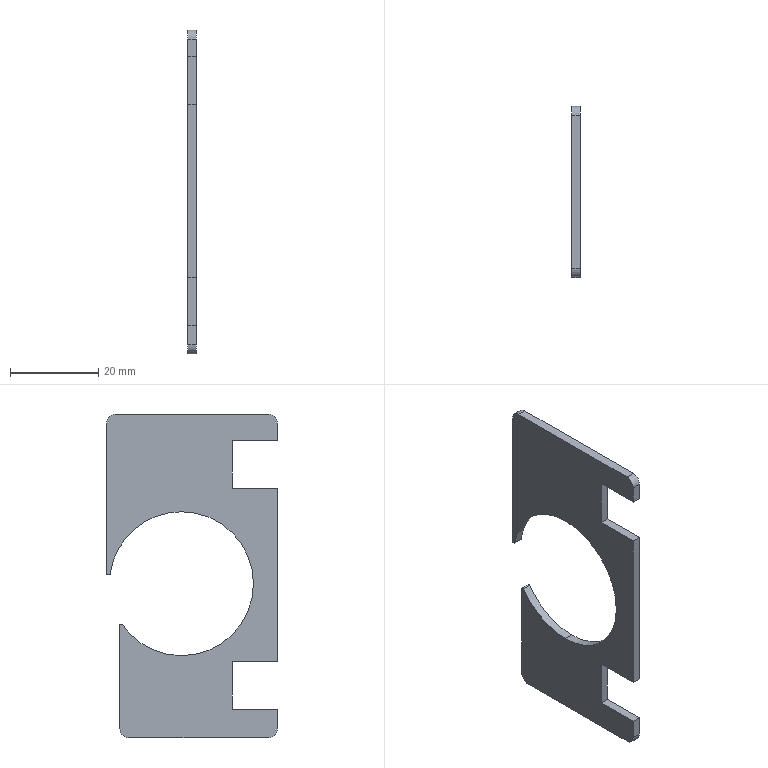Part | STEP file | ASND-0110-SDS_5 | 1 solid | 26 faces | box 2 x 38.8 x 73.5 mm | volume 3386 mm3 | plane 16 | cylinder 10 | commonest cylinder face diameters 4 x4 0.6 x3 32.7 x3